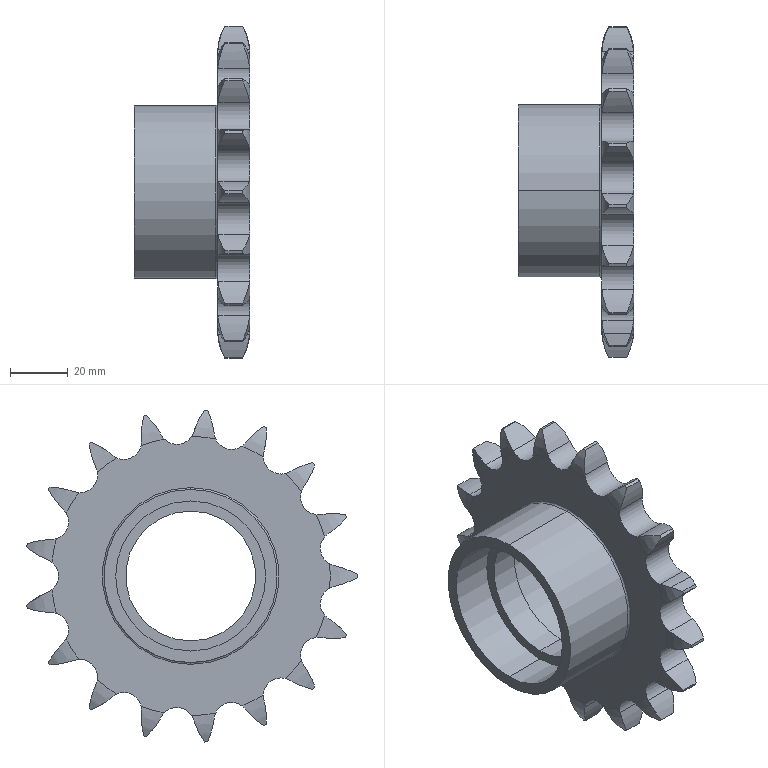Part | SolidWorks | features ICE 6, BaseBody 1, Fillet 1, RevCut 1 | 1 solid | 124 faces | box 40.001 x 114.527 x 115.015 mm | volume 88527 mm3 | cylinder 83 | spline 34 | plane 5 | torus 2 | commonest cylinder face diameters 55.039 x35 12.191 x23 115.416 x17 52 x4 45 x2 60 x2